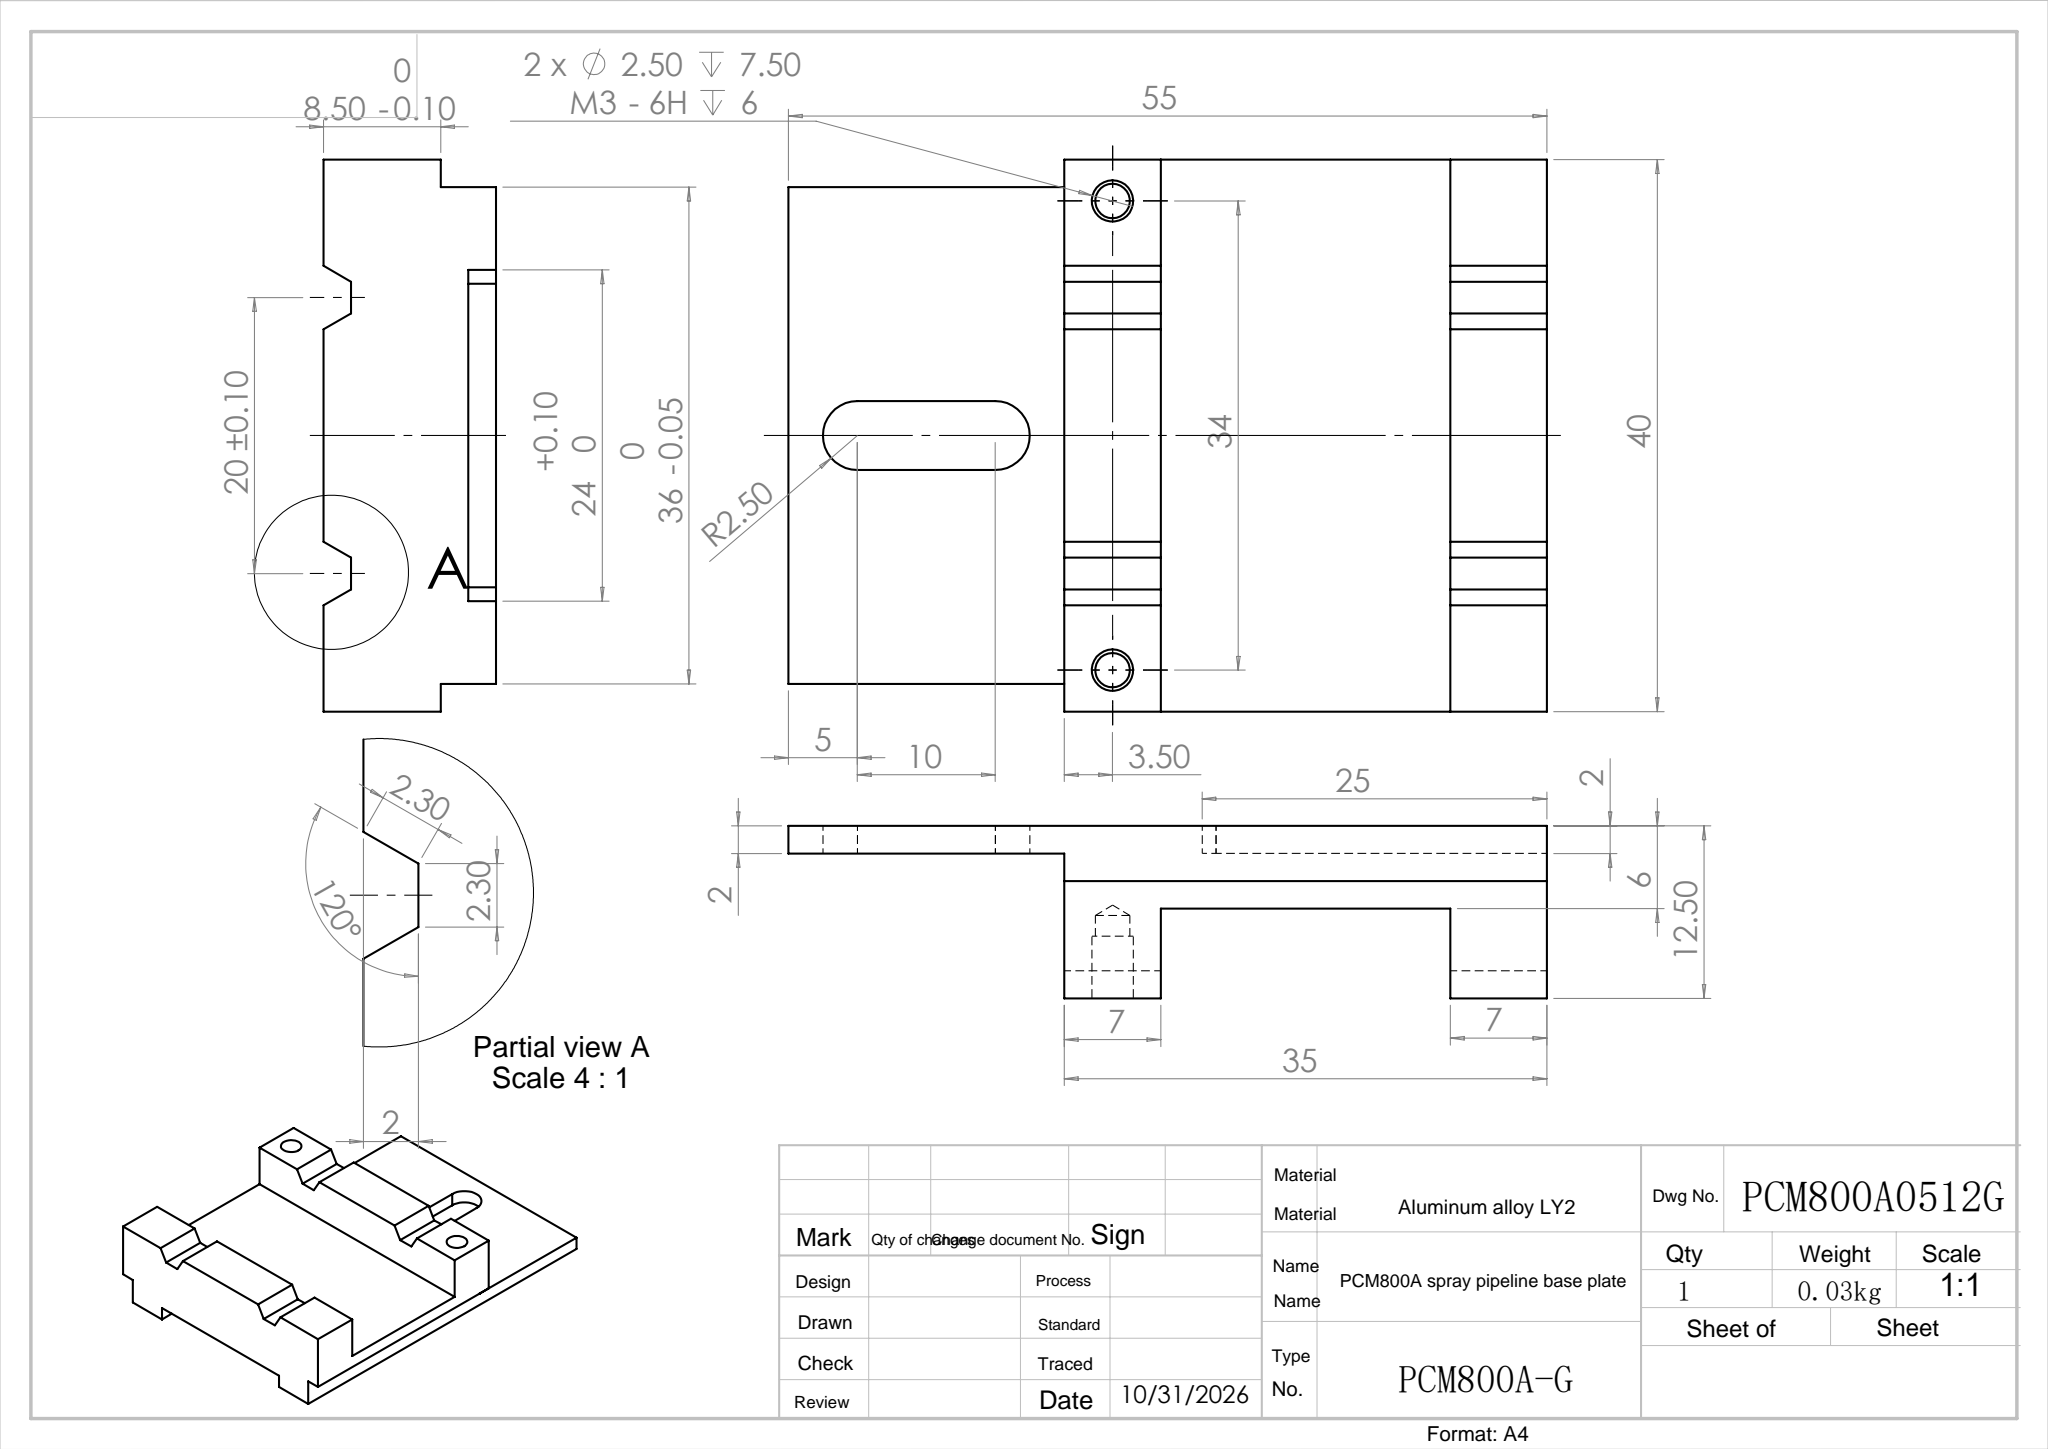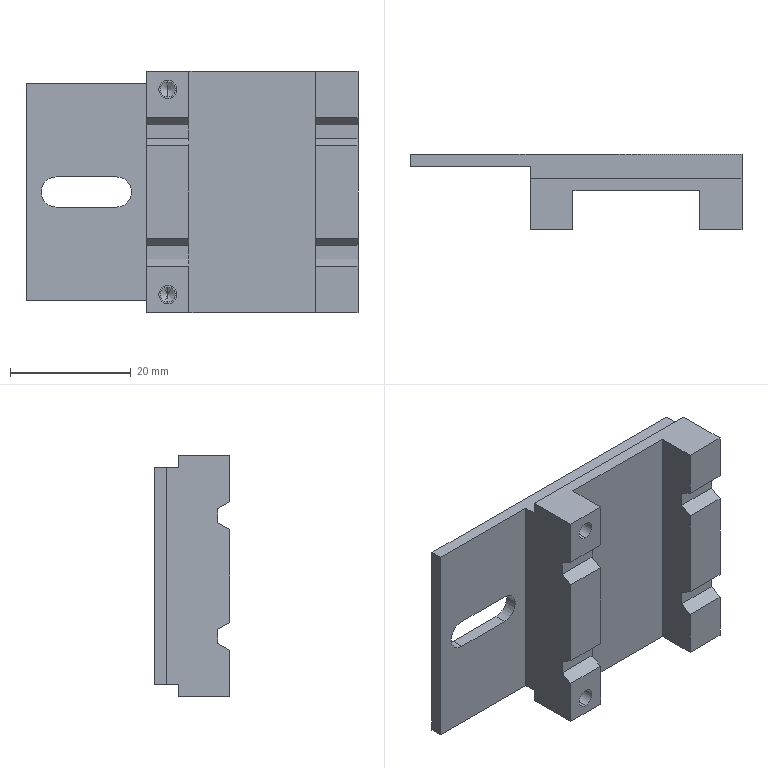Part | SolidWorks | features Boss 3, Cut 3, Extrusion 1, Fillet 1, HoleWzd 1, ICE 1, MirrorPattern 1 | 1 solid | 56 faces | box 55 x 12.5 x 40 mm | volume 11308 mm3 | plane 40 | cylinder 12 | cone 4 | commonest cylinder face diameters 2.5 x4 3 x4 2 x2 5 x2